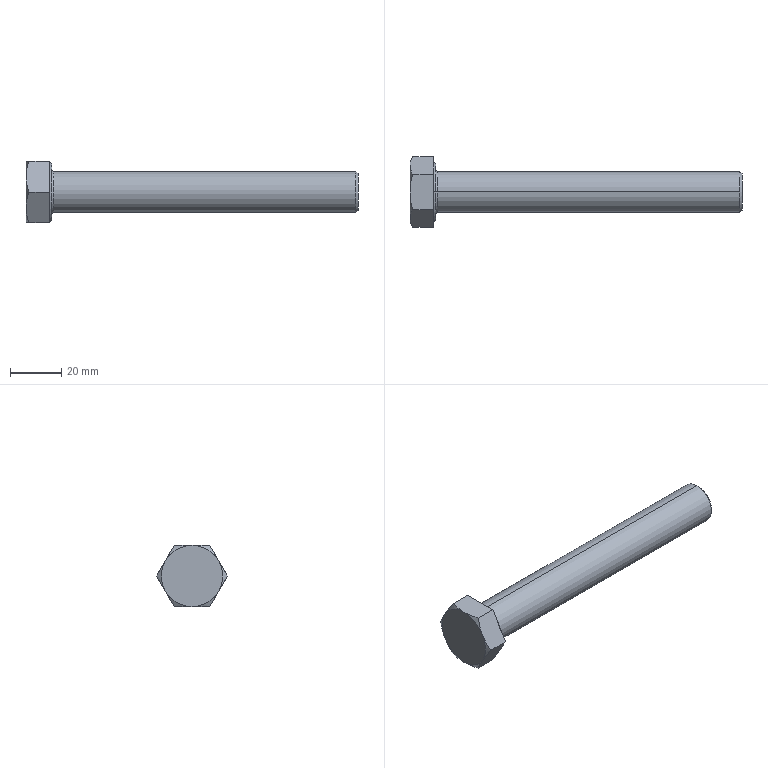Part | SolidWorks | features Chamfer 2, RevCut 2, Revolution 2, Extrusion 1, ICE 1 | 1 solid | 24 faces | box 130 x 27.713 x 24 mm | volume 29026 mm3 | cone 10 | plane 10 | cylinder 2 | torus 2 | commonest cylinder face diameters 16 x2
STEP:
#1=CARTESIAN_POINT('',(10.,0.,11.145));
#2=VERTEX_POINT('',#1);
#3=CARTESIAN_POINT('',(10.,0.,-11.145));
#4=VERTEX_POINT('',#3);
#5=CARTESIAN_POINT('',(10.,0.,0.));
#6=DIRECTION('',(-1.,0.,0.));
#7=DIRECTION('',(0.,0.,1.));
#8=AXIS2_PLACEMENT_3D('',#5,#6,#7);
#9=CIRCLE('',#8,11.145);
#10=EDGE_CURVE('',#2,#4,#9,.T.);
#11=ORIENTED_EDGE('',*,*,#10,.T.);
#12=CARTESIAN_POINT('',(9.2,0.,-11.945));
#13=VERTEX_POINT('',#12);
#14=CARTESIAN_POINT('',(9.2,0.,-11.945));
#15=DIRECTION('',(-0.7071,0.,-0.7071));
#16=VECTOR('',#15,1000.);
#17=LINE('',#14,#16);
#18=EDGE_CURVE('',#4,#13,#17,.T.);
#19=ORIENTED_EDGE('',*,*,#18,.T.);
#20=CARTESIAN_POINT('',(9.2,0.,11.945));
#21=VERTEX_POINT('',#20);
#22=CARTESIAN_POINT('',(9.2,0.,0.));
#23=DIRECTION('',(-1.,0.,0.));
#24=DIRECTION('',(0.,0.,1.));
#25=AXIS2_PLACEMENT_3D('',#22,#23,#24);
#26=CIRCLE('',#25,11.945);
#27=EDGE_CURVE('',#21,#13,#26,.T.);
#28=ORIENTED_EDGE('',*,*,#27,.F.);
#29=CARTESIAN_POINT('',(9.2,0.,11.945));
#30=DIRECTION('',(-0.7071,0.,0.7071));
#31=VECTOR('',#30,1000.);
#32=LINE('',#29,#31);
#33=EDGE_CURVE('',#2,#21,#32,.T.);
#34=ORIENTED_EDGE('',*,*,#33,.F.);
#35=EDGE_LOOP('',(#11,#19,#28,#34));
#36=FACE_OUTER_BOUND('',#35,.T.);
#37=CARTESIAN_POINT('',(9.2,0.,0.));
#38=DIRECTION('',(-1.,0.,0.));
#39=DIRECTION('',(0.,0.,1.));
#40=AXIS2_PLACEMENT_3D('',#37,#38,#39);
#41=CONICAL_SURFACE('',#40,11.945,0.7854);
#42=ADVANCED_FACE('',(#36),#41,.T.);
#43=CARTESIAN_POINT('',(130.,0.,-7.111));
#44=VERTEX_POINT('',#43);
#45=CARTESIAN_POINT('',(130.,0.,7.111));
#46=VERTEX_POINT('',#45);
#47=CARTESIAN_POINT('',(130.,0.,0.));
#48=DIRECTION('',(1.,0.,0.));
#49=DIRECTION('',(0.,0.,1.));
#50=AXIS2_PLACEMENT_3D('',#47,#48,#49);
#51=CIRCLE('',#50,7.111);
#52=EDGE_CURVE('',#44,#46,#51,.T.);
#53=ORIENTED_EDGE('',*,*,#52,.F.);
#54=CARTESIAN_POINT('',(129.111,0.,-8.));
#55=VERTEX_POINT('',#54);
#56=CARTESIAN_POINT('',(129.111,0.,-8.));
#57=DIRECTION('',(-0.7071,0.,-0.7071));
#58=VECTOR('',#57,1000.);
#59=LINE('',#56,#58);
#60=EDGE_CURVE('',#44,#55,#59,.T.);
#61=ORIENTED_EDGE('',*,*,#60,.T.);
#62=CARTESIAN_POINT('',(129.111,0.,8.));
#63=VERTEX_POINT('',#62);
#64=CARTESIAN_POINT('',(129.111,0.,0.));
#65=DIRECTION('',(-1.,0.,0.));
#66=DIRECTION('',(0.,0.,1.));
#67=AXIS2_PLACEMENT_3D('',#64,#65,#66);
#68=CIRCLE('',#67,8.);
#69=EDGE_CURVE('',#63,#55,#68,.T.);
#70=ORIENTED_EDGE('',*,*,#69,.F.);
#71=CARTESIAN_POINT('',(129.111,0.,8.));
#72=DIRECTION('',(-0.7071,0.,0.7071));
#73=VECTOR('',#72,1000.);
#74=LINE('',#71,#73);
#75=EDGE_CURVE('',#46,#63,#74,.T.);
#76=ORIENTED_EDGE('',*,*,#75,.F.);
#77=EDGE_LOOP('',(#53,#61,#70,#76));
#78=FACE_OUTER_BOUND('',#77,.T.);
#79=CARTESIAN_POINT('',(129.111,0.,0.));
#80=DIRECTION('',(-1.,0.,0.));
#81=DIRECTION('',(0.,0.,1.));
#82=AXIS2_PLACEMENT_3D('',#79,#80,#81);
#83=CONICAL_SURFACE('',#82,8.,0.7854);
#84=ADVANCED_FACE('',(#78),#83,.T.);
#85=ORIENTED_EDGE('',*,*,#69,.T.);
#86=CARTESIAN_POINT('',(10.85,0.,-8.));
#87=VERTEX_POINT('',#86);
#88=CARTESIAN_POINT('',(10.,0.,-8.));
#89=DIRECTION('',(-1.,0.,0.));
#90=VECTOR('',#89,1000.);
#91=LINE('',#88,#90);
#92=EDGE_CURVE('',#55,#87,#91,.T.);
#93=ORIENTED_EDGE('',*,*,#92,.T.);
#94=CARTESIAN_POINT('',(10.85,0.,8.));
#95=VERTEX_POINT('',#94);
#96=CARTESIAN_POINT('',(10.85,0.,0.));
#97=DIRECTION('',(-1.,0.,0.));
#98=DIRECTION('',(0.,0.,1.));
#99=AXIS2_PLACEMENT_3D('',#96,#97,#98);
#100=CIRCLE('',#99,8.);
#101=EDGE_CURVE('',#95,#87,#100,.T.);
#102=ORIENTED_EDGE('',*,*,#101,.F.);
#103=CARTESIAN_POINT('',(10.,0.,8.));
#104=DIRECTION('',(-1.,0.,0.));
#105=VECTOR('',#104,1000.);
#106=LINE('',#103,#105);
#107=EDGE_CURVE('',#63,#95,#106,.T.);
#108=ORIENTED_EDGE('',*,*,#107,.F.);
#109=EDGE_LOOP('',(#85,#93,#102,#108));
#110=FACE_OUTER_BOUND('',#109,.T.);
#111=CARTESIAN_POINT('',(10.,0.,0.));
#112=DIRECTION('',(-1.,0.,0.));
#113=DIRECTION('',(0.,0.,1.));
#114=AXIS2_PLACEMENT_3D('',#111,#112,#113);
#115=CYLINDRICAL_SURFACE('',#114,8.);
#116=ADVANCED_FACE('',(#110),#115,.T.);
#117=CARTESIAN_POINT('',(10.,0.,-8.85));
#118=VERTEX_POINT('',#117);
#119=CARTESIAN_POINT('',(10.,0.,8.85));
#120=VERTEX_POINT('',#119);
#121=CARTESIAN_POINT('',(10.,0.,0.));
#122=DIRECTION('',(-1.,0.,0.));
#123=DIRECTION('',(0.,0.,1.));
#124=AXIS2_PLACEMENT_3D('',#121,#122,#123);
#125=CIRCLE('',#124,8.85);
#126=EDGE_CURVE('',#118,#120,#125,.T.);
#127=ORIENTED_EDGE('',*,*,#126,.F.);
#128=CARTESIAN_POINT('',(10.85,0.,-8.85));
#129=DIRECTION('',(0.,1.,0.));
#130=DIRECTION('',(0.,0.,1.));
#131=AXIS2_PLACEMENT_3D('',#128,#129,#130);
#132=CIRCLE('',#131,0.85);
#133=EDGE_CURVE('',#118,#87,#132,.T.);
#134=ORIENTED_EDGE('',*,*,#133,.T.);
#135=CARTESIAN_POINT('',(10.85,0.,0.));
#136=DIRECTION('',(-1.,0.,0.));
#137=DIRECTION('',(0.,0.,1.));
#138=AXIS2_PLACEMENT_3D('',#135,#136,#137);
#139=CIRCLE('',#138,8.);
#140=EDGE_CURVE('',#87,#95,#139,.T.);
#141=ORIENTED_EDGE('',*,*,#140,.T.);
#142=CARTESIAN_POINT('',(10.85,0.,8.85));
#143=DIRECTION('',(0.,-1.,0.));
#144=DIRECTION('',(0.,0.,-1.));
#145=AXIS2_PLACEMENT_3D('',#142,#143,#144);
#146=CIRCLE('',#145,0.85);
#147=EDGE_CURVE('',#120,#95,#146,.T.);
#148=ORIENTED_EDGE('',*,*,#147,.F.);
#149=EDGE_LOOP('',(#127,#134,#141,#148));
#150=FACE_OUTER_BOUND('',#149,.T.);
#151=CARTESIAN_POINT('',(10.85,0.,0.));
#152=DIRECTION('',(-1.,0.,0.));
#153=DIRECTION('',(0.,0.,1.));
#154=AXIS2_PLACEMENT_3D('',#151,#152,#153);
#155=TOROIDAL_SURFACE('',#154,8.85,0.85);
#156=ADVANCED_FACE('',(#150),#155,.F.);
#157=CARTESIAN_POINT('',(10.,0.,0.));
#158=DIRECTION('',(-1.,0.,0.));
#159=DIRECTION('',(0.,0.,1.));
#160=AXIS2_PLACEMENT_3D('',#157,#158,#159);
#161=CIRCLE('',#160,8.85);
#162=EDGE_CURVE('',#120,#118,#161,.T.);
#163=ORIENTED_EDGE('',*,*,#162,.T.);
#164=ORIENTED_EDGE('',*,*,#126,.T.);
#165=EDGE_LOOP('',(#163,#164));
#166=FACE_BOUND('',#165,.T.);
#167=ORIENTED_EDGE('',*,*,#10,.F.);
#168=CARTESIAN_POINT('',(10.,0.,0.));
#169=DIRECTION('',(-1.,0.,0.));
#170=DIRECTION('',(0.,0.,1.));
#171=AXIS2_PLACEMENT_3D('',#168,#169,#170);
#172=CIRCLE('',#171,11.145);
#173=EDGE_CURVE('',#4,#2,#172,.T.);
#174=ORIENTED_EDGE('',*,*,#173,.F.);
#175=EDGE_LOOP('',(#167,#174));
#176=FACE_OUTER_BOUND('',#175,.T.);
#177=CARTESIAN_POINT('',(10.,6.928,-12.));
#178=DIRECTION('',(1.,0.,0.));
#179=DIRECTION('',(0.,0.,-1.));
#180=AXIS2_PLACEMENT_3D('',#177,#178,#179);
#181=PLANE('',#180);
#182=ADVANCED_FACE('',(#166,#176),#181,.T.);
#183=ORIENTED_EDGE('',*,*,#133,.F.);
#184=ORIENTED_EDGE('',*,*,#162,.F.);
#185=ORIENTED_EDGE('',*,*,#147,.T.);
#186=ORIENTED_EDGE('',*,*,#101,.T.);
#187=EDGE_LOOP('',(#183,#184,#185,#186));
#188=FACE_OUTER_BOUND('',#187,.T.);
#189=CARTESIAN_POINT('',(10.85,0.,0.));
#190=DIRECTION('',(-1.,0.,0.));
#191=DIRECTION('',(0.,0.,1.));
#192=AXIS2_PLACEMENT_3D('',#189,#190,#191);
#193=TOROIDAL_SURFACE('',#192,8.85,0.85);
#194=ADVANCED_FACE('',(#188),#193,.F.);
#195=CARTESIAN_POINT('',(130.,0.,0.));
#196=DIRECTION('',(1.,0.,0.));
#197=DIRECTION('',(0.,0.,1.));
#198=AXIS2_PLACEMENT_3D('',#195,#196,#197);
#199=CIRCLE('',#198,7.111);
#200=EDGE_CURVE('',#46,#44,#199,.T.);
#201=ORIENTED_EDGE('',*,*,#200,.T.);
#202=ORIENTED_EDGE('',*,*,#52,.T.);
#203=EDGE_LOOP('',(#201,#202));
#204=FACE_OUTER_BOUND('',#203,.T.);
#205=CARTESIAN_POINT('',(130.,8.,0.));
#206=DIRECTION('',(-1.,0.,0.));
#207=DIRECTION('',(0.,0.,1.));
#208=AXIS2_PLACEMENT_3D('',#205,#206,#207);
#209=PLANE('',#208);
#210=ADVANCED_FACE('',(#204),#209,.F.);
#211=ORIENTED_EDGE('',*,*,#92,.F.);
#212=CARTESIAN_POINT('',(129.111,0.,0.));
#213=DIRECTION('',(-1.,0.,0.));
#214=DIRECTION('',(0.,0.,1.));
#215=AXIS2_PLACEMENT_3D('',#212,#213,#214);
#216=CIRCLE('',#215,8.);
#217=EDGE_CURVE('',#55,#63,#216,.T.);
#218=ORIENTED_EDGE('',*,*,#217,.T.);
#219=ORIENTED_EDGE('',*,*,#107,.T.);
#220=ORIENTED_EDGE('',*,*,#140,.F.);
#221=EDGE_LOOP('',(#211,#218,#219,#220));
#222=FACE_OUTER_BOUND('',#221,.T.);
#223=CARTESIAN_POINT('',(10.,0.,0.));
#224=DIRECTION('',(-1.,0.,0.));
#225=DIRECTION('',(0.,0.,1.));
#226=AXIS2_PLACEMENT_3D('',#223,#224,#225);
#227=CYLINDRICAL_SURFACE('',#226,8.);
#228=ADVANCED_FACE('',(#222),#227,.T.);
#229=ORIENTED_EDGE('',*,*,#60,.F.);
#230=ORIENTED_EDGE('',*,*,#200,.F.);
#231=ORIENTED_EDGE('',*,*,#75,.T.);
#232=ORIENTED_EDGE('',*,*,#217,.F.);
#233=EDGE_LOOP('',(#229,#230,#231,#232));
#234=FACE_OUTER_BOUND('',#233,.T.);
#235=CARTESIAN_POINT('',(129.111,0.,0.));
#236=DIRECTION('',(-1.,0.,0.));
#237=DIRECTION('',(0.,0.,1.));
#238=AXIS2_PLACEMENT_3D('',#235,#236,#237);
#239=CONICAL_SURFACE('',#238,8.,0.7854);
#240=ADVANCED_FACE('',(#234),#239,.T.);
#241=ORIENTED_EDGE('',*,*,#27,.T.);
#242=CARTESIAN_POINT('',(9.2,0.,0.));
#243=DIRECTION('',(-1.,0.,0.));
#244=DIRECTION('',(0.,0.,1.));
#245=AXIS2_PLACEMENT_3D('',#242,#243,#244);
#246=CIRCLE('',#245,11.945);
#247=EDGE_CURVE('',#13,#21,#246,.T.);
#248=ORIENTED_EDGE('',*,*,#247,.T.);
#249=EDGE_LOOP('',(#241,#248));
#250=FACE_BOUND('',#249,.T.);
#251=CARTESIAN_POINT('',(9.2,-6.928,-12.));
#252=VERTEX_POINT('',#251);
#253=CARTESIAN_POINT('',(9.2,6.928,-12.));
#254=VERTEX_POINT('',#253);
#255=CARTESIAN_POINT('',(9.2,-6.928,-12.));
#256=DIRECTION('',(0.,1.,0.));
#257=VECTOR('',#256,1000.);
#258=LINE('',#255,#257);
#259=EDGE_CURVE('',#252,#254,#258,.T.);
#260=ORIENTED_EDGE('',*,*,#259,.T.);
#261=CARTESIAN_POINT('',(9.2,13.856,0.));
#262=VERTEX_POINT('',#261);
#263=CARTESIAN_POINT('',(9.2,6.928,-12.));
#264=DIRECTION('',(0.,0.5,0.866));
#265=VECTOR('',#264,1000.);
#266=LINE('',#263,#265);
#267=EDGE_CURVE('',#254,#262,#266,.T.);
#268=ORIENTED_EDGE('',*,*,#267,.T.);
#269=CARTESIAN_POINT('',(9.2,6.928,12.));
#270=VERTEX_POINT('',#269);
#271=CARTESIAN_POINT('',(9.2,13.856,0.));
#272=DIRECTION('',(0.,-0.5,0.866));
#273=VECTOR('',#272,1000.);
#274=LINE('',#271,#273);
#275=EDGE_CURVE('',#262,#270,#274,.T.);
#276=ORIENTED_EDGE('',*,*,#275,.T.);
#277=CARTESIAN_POINT('',(9.2,-6.928,12.));
#278=VERTEX_POINT('',#277);
#279=CARTESIAN_POINT('',(9.2,6.928,12.));
#280=DIRECTION('',(0.,-1.,0.));
#281=VECTOR('',#280,1000.);
#282=LINE('',#279,#281);
#283=EDGE_CURVE('',#270,#278,#282,.T.);
#284=ORIENTED_EDGE('',*,*,#283,.T.);
#285=CARTESIAN_POINT('',(9.2,-13.856,0.));
#286=VERTEX_POINT('',#285);
#287=CARTESIAN_POINT('',(9.2,-6.928,12.));
#288=DIRECTION('',(0.,-0.5,-0.866));
#289=VECTOR('',#288,1000.);
#290=LINE('',#287,#289);
#291=EDGE_CURVE('',#278,#286,#290,.T.);
#292=ORIENTED_EDGE('',*,*,#291,.T.);
#293=CARTESIAN_POINT('',(9.2,-13.856,0.));
#294=DIRECTION('',(0.,0.5,-0.866));
#295=VECTOR('',#294,1000.);
#296=LINE('',#293,#295);
#297=EDGE_CURVE('',#286,#252,#296,.T.);
#298=ORIENTED_EDGE('',*,*,#297,.T.);
#299=EDGE_LOOP('',(#260,#268,#276,#284,#292,#298));
#300=FACE_OUTER_BOUND('',#299,.T.);
#301=CARTESIAN_POINT('',(9.2,-11.945,0.));
#302=DIRECTION('',(1.,0.,0.));
#303=DIRECTION('',(0.,0.,-1.));
#304=AXIS2_PLACEMENT_3D('',#301,#302,#303);
#305=PLANE('',#304);
#306=ADVANCED_FACE('',(#250,#300),#305,.T.);
#307=ORIENTED_EDGE('',*,*,#18,.F.);
#308=ORIENTED_EDGE('',*,*,#173,.T.);
#309=ORIENTED_EDGE('',*,*,#33,.T.);
#310=ORIENTED_EDGE('',*,*,#247,.F.);
#311=EDGE_LOOP('',(#307,#308,#309,#310));
#312=FACE_OUTER_BOUND('',#311,.T.);
#313=CARTESIAN_POINT('',(9.2,0.,0.));
#314=DIRECTION('',(-1.,0.,0.));
#315=DIRECTION('',(0.,0.,1.));
#316=AXIS2_PLACEMENT_3D('',#313,#314,#315);
#317=CONICAL_SURFACE('',#316,11.945,0.7854);
#318=ADVANCED_FACE('',(#312),#317,.T.);
#319=CARTESIAN_POINT('',(0.,0.,-12.));
#320=VERTEX_POINT('',#319);
#321=CARTESIAN_POINT('',(0.,10.392,-6.));
#322=VERTEX_POINT('',#321);
#323=CARTESIAN_POINT('',(0.,0.,0.));
#324=DIRECTION('',(1.,0.,0.));
#325=DIRECTION('',(0.,0.,-1.));
#326=AXIS2_PLACEMENT_3D('',#323,#324,#325);
#327=CIRCLE('',#326,12.);
#328=EDGE_CURVE('',#320,#322,#327,.T.);
#329=ORIENTED_EDGE('',*,*,#328,.F.);
#330=CARTESIAN_POINT('',(0.,-10.392,-6.));
#331=VERTEX_POINT('',#330);
#332=CARTESIAN_POINT('',(0.,0.,0.));
#333=DIRECTION('',(1.,0.,0.));
#334=DIRECTION('',(0.,0.,-1.));
#335=AXIS2_PLACEMENT_3D('',#332,#333,#334);
#336=CIRCLE('',#335,12.);
#337=EDGE_CURVE('',#331,#320,#336,.T.);
#338=ORIENTED_EDGE('',*,*,#337,.F.);
#339=CARTESIAN_POINT('',(0.,-10.392,6.));
#340=VERTEX_POINT('',#339);
#341=CARTESIAN_POINT('',(0.,0.,0.));
#342=DIRECTION('',(1.,0.,0.));
#343=DIRECTION('',(0.,0.,-1.));
#344=AXIS2_PLACEMENT_3D('',#341,#342,#343);
#345=CIRCLE('',#344,12.);
#346=EDGE_CURVE('',#340,#331,#345,.T.);
#347=ORIENTED_EDGE('',*,*,#346,.F.);
#348=CARTESIAN_POINT('',(0.,0.,12.));
#349=VERTEX_POINT('',#348);
#350=CARTESIAN_POINT('',(0.,0.,0.));
#351=DIRECTION('',(1.,0.,0.));
#352=DIRECTION('',(0.,0.,-1.));
#353=AXIS2_PLACEMENT_3D('',#350,#351,#352);
#354=CIRCLE('',#353,12.);
#355=EDGE_CURVE('',#349,#340,#354,.T.);
#356=ORIENTED_EDGE('',*,*,#355,.F.);
#357=CARTESIAN_POINT('',(0.,10.392,6.));
#358=VERTEX_POINT('',#357);
#359=CARTESIAN_POINT('',(0.,0.,0.));
#360=DIRECTION('',(-1.,0.,0.));
#361=DIRECTION('',(0.,0.,1.));
#362=AXIS2_PLACEMENT_3D('',#359,#360,#361);
#363=CIRCLE('',#362,12.);
#364=EDGE_CURVE('',#349,#358,#363,.T.);
#365=ORIENTED_EDGE('',*,*,#364,.T.);
#366=CARTESIAN_POINT('',(0.,0.,0.));
#367=DIRECTION('',(1.,0.,0.));
#368=DIRECTION('',(0.,0.,-1.));
#369=AXIS2_PLACEMENT_3D('',#366,#367,#368);
#370=CIRCLE('',#369,12.);
#371=EDGE_CURVE('',#322,#358,#370,.T.);
#372=ORIENTED_EDGE('',*,*,#371,.F.);
#373=EDGE_LOOP('',(#329,#338,#347,#356,#365,#372));
#374=FACE_OUTER_BOUND('',#373,.T.);
#375=CARTESIAN_POINT('',(0.,6.928,-12.));
#376=DIRECTION('',(1.,0.,0.));
#377=DIRECTION('',(0.,0.,-1.));
#378=AXIS2_PLACEMENT_3D('',#375,#376,#377);
#379=PLANE('',#378);
#380=ADVANCED_FACE('',(#374),#379,.F.);
#381=CARTESIAN_POINT('',(1.072,6.928,-12.));
#382=VERTEX_POINT('',#381);
#383=CARTESIAN_POINT('',(0.,10.392,-6.));
#384=CARTESIAN_POINT('',(0.,10.098,-6.509));
#385=CARTESIAN_POINT('',(0.02533,9.803,-7.021));
#386=CARTESIAN_POINT('',(0.1234,9.219,-8.033));
#387=CARTESIAN_POINT('',(0.196,8.929,-8.535));
#388=CARTESIAN_POINT('',(0.476,8.063,-10.034));
#389=CARTESIAN_POINT('',(0.7454,7.493,-11.021));
#390=CARTESIAN_POINT('',(1.072,6.928,-12.));
#391=B_SPLINE_CURVE_WITH_KNOTS('',3,(#383,#384,#385,#386,#387,#388,#389,#390),.UNSPECIFIED.,.F.,.F.,(4,2,2,4),(0.00701,0.008756,0.0105,0.01399),.UNSPECIFIED.);
#392=EDGE_CURVE('',#322,#382,#391,.T.);
#393=ORIENTED_EDGE('',*,*,#392,.T.);
#394=CARTESIAN_POINT('',(1.072,6.928,-12.));
#395=CARTESIAN_POINT('',(0.7484,5.808,-12.));
#396=CARTESIAN_POINT('',(0.4791,4.673,-12.));
#397=CARTESIAN_POINT('',(0.1974,2.937,-12.));
#398=CARTESIAN_POINT('',(0.1238,2.353,-12.));
#399=CARTESIAN_POINT('',(0.0249,1.173,-12.));
#400=CARTESIAN_POINT('',(0.,0.5858,-12.));
#401=CARTESIAN_POINT('',(0.,0.,-12.));
#402=B_SPLINE_CURVE_WITH_KNOTS('',3,(#394,#395,#396,#397,#398,#399,#400,#401),.UNSPECIFIED.,.F.,.F.,(4,2,2,4),(0.005049,0.008547,0.0103,0.01204),.UNSPECIFIED.);
#403=EDGE_CURVE('',#382,#320,#402,.T.);
#404=ORIENTED_EDGE('',*,*,#403,.T.);
#405=ORIENTED_EDGE('',*,*,#328,.T.);
#406=EDGE_LOOP('',(#393,#404,#405));
#407=FACE_OUTER_BOUND('',#406,.T.);
#408=CARTESIAN_POINT('',(0.,0.,0.));
#409=DIRECTION('',(1.,0.,0.));
#410=DIRECTION('',(0.,0.,1.));
#411=AXIS2_PLACEMENT_3D('',#408,#409,#410);
#412=CONICAL_SURFACE('',#411,12.,1.047);
#413=ADVANCED_FACE('',(#407),#412,.T.);
#414=CARTESIAN_POINT('',(1.072,13.856,0.));
#415=VERTEX_POINT('',#414);
#416=CARTESIAN_POINT('',(0.,10.392,6.));
#417=CARTESIAN_POINT('',(0.,10.686,5.491));
#418=CARTESIAN_POINT('',(0.02533,10.982,4.979));
#419=CARTESIAN_POINT('',(0.1234,11.566,3.967));
#420=CARTESIAN_POINT('',(0.196,11.856,3.465));
#421=CARTESIAN_POINT('',(0.476,12.721,1.966));
#422=CARTESIAN_POINT('',(0.7454,13.291,0.9791));
#423=CARTESIAN_POINT('',(1.072,13.856,0.));
#424=B_SPLINE_CURVE_WITH_KNOTS('',3,(#416,#417,#418,#419,#420,#421,#422,#423),.UNSPECIFIED.,.F.,.F.,(4,2,2,4),(0.00701,0.008756,0.0105,0.01399),.UNSPECIFIED.);
#425=EDGE_CURVE('',#358,#415,#424,.T.);
#426=ORIENTED_EDGE('',*,*,#425,.T.);
#427=CARTESIAN_POINT('',(1.072,13.856,0.));
#428=CARTESIAN_POINT('',(0.7446,13.29,-0.9815));
#429=CARTESIAN_POINT('',(0.4751,12.719,-1.97));
#430=CARTESIAN_POINT('',(0.1021,11.565,-3.968));
#431=CARTESIAN_POINT('',(0.,10.982,-4.978));
#432=CARTESIAN_POINT('',(0.,10.392,-6.));
#433=B_SPLINE_CURVE_WITH_KNOTS('',3,(#427,#428,#429,#430,#431,#432),.UNSPECIFIED.,.F.,.F.,(4,2,4),(0.000000238,0.003505,0.00701),.UNSPECIFIED.);
#434=EDGE_CURVE('',#415,#322,#433,.T.);
#435=ORIENTED_EDGE('',*,*,#434,.T.);
#436=ORIENTED_EDGE('',*,*,#371,.T.);
#437=EDGE_LOOP('',(#426,#435,#436));
#438=FACE_OUTER_BOUND('',#437,.T.);
#439=CARTESIAN_POINT('',(0.,0.,0.));
#440=DIRECTION('',(1.,0.,0.));
#441=DIRECTION('',(0.,0.,1.));
#442=AXIS2_PLACEMENT_3D('',#439,#440,#441);
#443=CONICAL_SURFACE('',#442,12.,1.047);
#444=ADVANCED_FACE('',(#438),#443,.T.);
#445=CARTESIAN_POINT('',(1.072,6.928,12.));
#446=VERTEX_POINT('',#445);
#447=CARTESIAN_POINT('',(1.072,6.928,12.));
#448=CARTESIAN_POINT('',(0.7446,7.495,11.018));
#449=CARTESIAN_POINT('',(0.4751,8.066,10.03));
#450=CARTESIAN_POINT('',(0.1021,9.219,8.032));
#451=CARTESIAN_POINT('',(0.,9.802,7.022));
#452=CARTESIAN_POINT('',(0.,10.392,6.));
#453=B_SPLINE_CURVE_WITH_KNOTS('',3,(#447,#448,#449,#450,#451,#452),.UNSPECIFIED.,.F.,.F.,(4,2,4),(0.000000238,0.003505,0.00701),.UNSPECIFIED.);
#454=EDGE_CURVE('',#446,#358,#453,.T.);
#455=ORIENTED_EDGE('',*,*,#454,.T.);
#456=ORIENTED_EDGE('',*,*,#364,.F.);
#457=CARTESIAN_POINT('',(0.,0.,12.));
#458=CARTESIAN_POINT('',(0.,0.5858,12.));
#459=CARTESIAN_POINT('',(0.0249,1.173,12.));
#460=CARTESIAN_POINT('',(0.1238,2.353,12.));
#461=CARTESIAN_POINT('',(0.1974,2.937,12.));
#462=CARTESIAN_POINT('',(0.4791,4.673,12.));
#463=CARTESIAN_POINT('',(0.7484,5.808,12.));
#464=CARTESIAN_POINT('',(1.072,6.928,12.));
#465=B_SPLINE_CURVE_WITH_KNOTS('',3,(#457,#458,#459,#460,#461,#462,#463,#464),.UNSPECIFIED.,.F.,.F.,(4,2,2,4),(0.0194,0.02115,0.0229,0.02641),.UNSPECIFIED.);
#466=EDGE_CURVE('',#349,#446,#465,.T.);
#467=ORIENTED_EDGE('',*,*,#466,.T.);
#468=EDGE_LOOP('',(#455,#456,#467));
#469=FACE_OUTER_BOUND('',#468,.T.);
#470=CARTESIAN_POINT('',(0.,0.,0.));
#471=DIRECTION('',(1.,0.,0.));
#472=DIRECTION('',(0.,0.,1.));
#473=AXIS2_PLACEMENT_3D('',#470,#471,#472);
#474=CONICAL_SURFACE('',#473,12.,1.047);
#475=ADVANCED_FACE('',(#469),#474,.T.);
#476=CARTESIAN_POINT('',(1.072,-6.928,12.));
#477=VERTEX_POINT('',#476);
#478=CARTESIAN_POINT('',(1.072,-6.928,12.));
#479=CARTESIAN_POINT('',(0.7465,-5.801,12.));
#480=CARTESIAN_POINT('',(0.4737,-4.647,12.));
#481=CARTESIAN_POINT('',(0.1006,-2.334,12.));
#482=CARTESIAN_POINT('',(0.,-1.171,12.));
#483=CARTESIAN_POINT('',(0.,0.,12.));
#484=B_SPLINE_CURVE_WITH_KNOTS('',3,(#478,#479,#480,#481,#482,#483),.UNSPECIFIED.,.F.,.F.,(4,2,4),(0.01239,0.01589,0.0194),.UNSPECIFIED.);
#485=EDGE_CURVE('',#477,#349,#484,.T.);
#486=ORIENTED_EDGE('',*,*,#485,.T.);
#487=ORIENTED_EDGE('',*,*,#355,.T.);
#488=CARTESIAN_POINT('',(0.,-10.392,6.));
#489=CARTESIAN_POINT('',(0.,-10.098,6.509));
#490=CARTESIAN_POINT('',(0.02533,-9.803,7.021));
#491=CARTESIAN_POINT('',(0.1234,-9.219,8.033));
#492=CARTESIAN_POINT('',(0.196,-8.929,8.535));
#493=CARTESIAN_POINT('',(0.476,-8.063,10.034));
#494=CARTESIAN_POINT('',(0.7454,-7.493,11.021));
#495=CARTESIAN_POINT('',(1.072,-6.928,12.));
#496=B_SPLINE_CURVE_WITH_KNOTS('',3,(#488,#489,#490,#491,#492,#493,#494,#495),.UNSPECIFIED.,.F.,.F.,(4,2,2,4),(0.00701,0.008756,0.0105,0.01399),.UNSPECIFIED.);
#497=EDGE_CURVE('',#340,#477,#496,.T.);
#498=ORIENTED_EDGE('',*,*,#497,.T.);
#499=EDGE_LOOP('',(#486,#487,#498));
#500=FACE_OUTER_BOUND('',#499,.T.);
#501=CARTESIAN_POINT('',(0.,0.,0.));
#502=DIRECTION('',(1.,0.,0.));
#503=DIRECTION('',(0.,0.,1.));
#504=AXIS2_PLACEMENT_3D('',#501,#502,#503);
#505=CONICAL_SURFACE('',#504,12.,1.047);
#506=ADVANCED_FACE('',(#500),#505,.T.);
#507=CARTESIAN_POINT('',(1.072,-6.928,-12.));
#508=VERTEX_POINT('',#507);
#509=CARTESIAN_POINT('',(0.,0.,-12.));
#510=CARTESIAN_POINT('',(0.,-1.171,-12.));
#511=CARTESIAN_POINT('',(0.1006,-2.334,-12.));
#512=CARTESIAN_POINT('',(0.4737,-4.647,-12.));
#513=CARTESIAN_POINT('',(0.7465,-5.801,-12.));
#514=CARTESIAN_POINT('',(1.072,-6.928,-12.));
#515=B_SPLINE_CURVE_WITH_KNOTS('',3,(#509,#510,#511,#512,#513,#514),.UNSPECIFIED.,.F.,.F.,(4,2,4),(0.01204,0.01554,0.01904),.UNSPECIFIED.);
#516=EDGE_CURVE('',#320,#508,#515,.T.);
#517=ORIENTED_EDGE('',*,*,#516,.T.);
#518=CARTESIAN_POINT('',(1.072,-6.928,-12.));
#519=CARTESIAN_POINT('',(0.7446,-7.495,-11.018));
#520=CARTESIAN_POINT('',(0.4751,-8.066,-10.03));
#521=CARTESIAN_POINT('',(0.1021,-9.219,-8.032));
#522=CARTESIAN_POINT('',(0.,-9.802,-7.022));
#523=CARTESIAN_POINT('',(0.,-10.392,-6.));
#524=B_SPLINE_CURVE_WITH_KNOTS('',3,(#518,#519,#520,#521,#522,#523),.UNSPECIFIED.,.F.,.F.,(4,2,4),(0.000000238,0.003505,0.00701),.UNSPECIFIED.);
#525=EDGE_CURVE('',#508,#331,#524,.T.);
#526=ORIENTED_EDGE('',*,*,#525,.T.);
#527=ORIENTED_EDGE('',*,*,#337,.T.);
#528=EDGE_LOOP('',(#517,#526,#527));
#529=FACE_OUTER_BOUND('',#528,.T.);
#530=CARTESIAN_POINT('',(0.,0.,0.));
#531=DIRECTION('',(1.,0.,0.));
#532=DIRECTION('',(0.,0.,1.));
#533=AXIS2_PLACEMENT_3D('',#530,#531,#532);
#534=CONICAL_SURFACE('',#533,12.,1.047);
#535=ADVANCED_FACE('',(#529),#534,.T.);
#536=CARTESIAN_POINT('',(1.072,-13.856,0.));
#537=VERTEX_POINT('',#536);
#538=CARTESIAN_POINT('',(1.072,-13.856,0.));
#539=CARTESIAN_POINT('',(0.7446,-13.29,0.9815));
#540=CARTESIAN_POINT('',(0.4751,-12.719,1.97));
#541=CARTESIAN_POINT('',(0.1021,-11.565,3.968));
#542=CARTESIAN_POINT('',(0.,-10.982,4.978));
#543=CARTESIAN_POINT('',(0.,-10.392,6.));
#544=B_SPLINE_CURVE_WITH_KNOTS('',3,(#538,#539,#540,#541,#542,#543),.UNSPECIFIED.,.F.,.F.,(4,2,4),(0.000000238,0.003505,0.00701),.UNSPECIFIED.);
#545=EDGE_CURVE('',#537,#340,#544,.T.);
#546=ORIENTED_EDGE('',*,*,#545,.T.);
#547=ORIENTED_EDGE('',*,*,#346,.T.);
#548=CARTESIAN_POINT('',(0.,-10.392,-6.));
#549=CARTESIAN_POINT('',(0.,-10.686,-5.491));
#550=CARTESIAN_POINT('',(0.02533,-10.982,-4.979));
#551=CARTESIAN_POINT('',(0.1234,-11.566,-3.967));
#552=CARTESIAN_POINT('',(0.196,-11.856,-3.465));
#553=CARTESIAN_POINT('',(0.476,-12.721,-1.966));
#554=CARTESIAN_POINT('',(0.7454,-13.291,-0.9791));
#555=CARTESIAN_POINT('',(1.072,-13.856,0.));
#556=B_SPLINE_CURVE_WITH_KNOTS('',3,(#548,#549,#550,#551,#552,#553,#554,#555),.UNSPECIFIED.,.F.,.F.,(4,2,2,4),(0.00701,0.008756,0.0105,0.01399),.UNSPECIFIED.);
#557=EDGE_CURVE('',#331,#537,#556,.T.);
#558=ORIENTED_EDGE('',*,*,#557,.T.);
#559=EDGE_LOOP('',(#546,#547,#558));
#560=FACE_OUTER_BOUND('',#559,.T.);
#561=CARTESIAN_POINT('',(0.,0.,0.));
#562=DIRECTION('',(1.,0.,0.));
#563=DIRECTION('',(0.,0.,1.));
#564=AXIS2_PLACEMENT_3D('',#561,#562,#563);
#565=CONICAL_SURFACE('',#564,12.,1.047);
#566=ADVANCED_FACE('',(#560),#565,.T.);
#567=ORIENTED_EDGE('',*,*,#297,.F.);
#568=CARTESIAN_POINT('',(10.,-13.856,0.));
#569=DIRECTION('',(-1.,0.,0.));
#570=VECTOR('',#569,1000.);
#571=LINE('',#568,#570);
#572=EDGE_CURVE('',#286,#537,#571,.T.);
#573=ORIENTED_EDGE('',*,*,#572,.T.);
#574=ORIENTED_EDGE('',*,*,#557,.F.);
#575=ORIENTED_EDGE('',*,*,#525,.F.);
#576=CARTESIAN_POINT('',(10.,-6.928,-12.));
#577=DIRECTION('',(-1.,0.,0.));
#578=VECTOR('',#577,1000.);
#579=LINE('',#576,#578);
#580=EDGE_CURVE('',#252,#508,#579,.T.);
#581=ORIENTED_EDGE('',*,*,#580,.F.);
#582=EDGE_LOOP('',(#567,#573,#574,#575,#581));
#583=FACE_OUTER_BOUND('',#582,.T.);
#584=CARTESIAN_POINT('',(10.,-13.856,0.));
#585=DIRECTION('',(0.,0.866,0.5));
#586=DIRECTION('',(0.,-0.5,0.866));
#587=AXIS2_PLACEMENT_3D('',#584,#585,#586);
#588=PLANE('',#587);
#589=ADVANCED_FACE('',(#583),#588,.F.);
#590=ORIENTED_EDGE('',*,*,#291,.F.);
#591=CARTESIAN_POINT('',(10.,-6.928,12.));
#592=DIRECTION('',(-1.,0.,0.));
#593=VECTOR('',#592,1000.);
#594=LINE('',#591,#593);
#595=EDGE_CURVE('',#278,#477,#594,.T.);
#596=ORIENTED_EDGE('',*,*,#595,.T.);
#597=ORIENTED_EDGE('',*,*,#497,.F.);
#598=ORIENTED_EDGE('',*,*,#545,.F.);
#599=ORIENTED_EDGE('',*,*,#572,.F.);
#600=EDGE_LOOP('',(#590,#596,#597,#598,#599));
#601=FACE_OUTER_BOUND('',#600,.T.);
#602=CARTESIAN_POINT('',(10.,-6.928,12.));
#603=DIRECTION('',(0.,0.866,-0.5));
#604=DIRECTION('',(0.,0.5,0.866));
#605=AXIS2_PLACEMENT_3D('',#602,#603,#604);
#606=PLANE('',#605);
#607=ADVANCED_FACE('',(#601),#606,.F.);
#608=ORIENTED_EDGE('',*,*,#283,.F.);
#609=CARTESIAN_POINT('',(10.,6.928,12.));
#610=DIRECTION('',(-1.,0.,0.));
#611=VECTOR('',#610,1000.);
#612=LINE('',#609,#611);
#613=EDGE_CURVE('',#270,#446,#612,.T.);
#614=ORIENTED_EDGE('',*,*,#613,.T.);
#615=ORIENTED_EDGE('',*,*,#466,.F.);
#616=ORIENTED_EDGE('',*,*,#485,.F.);
#617=ORIENTED_EDGE('',*,*,#595,.F.);
#618=EDGE_LOOP('',(#608,#614,#615,#616,#617));
#619=FACE_OUTER_BOUND('',#618,.T.);
#620=CARTESIAN_POINT('',(10.,6.928,12.));
#621=DIRECTION('',(0.,0.,-1.));
#622=DIRECTION('',(0.,1.,0.));
#623=AXIS2_PLACEMENT_3D('',#620,#621,#622);
#624=PLANE('',#623);
#625=ADVANCED_FACE('',(#619),#624,.F.);
#626=ORIENTED_EDGE('',*,*,#275,.F.);
#627=CARTESIAN_POINT('',(10.,13.856,0.));
#628=DIRECTION('',(-1.,0.,0.));
#629=VECTOR('',#628,1000.);
#630=LINE('',#627,#629);
#631=EDGE_CURVE('',#262,#415,#630,.T.);
#632=ORIENTED_EDGE('',*,*,#631,.T.);
#633=ORIENTED_EDGE('',*,*,#425,.F.);
#634=ORIENTED_EDGE('',*,*,#454,.F.);
#635=ORIENTED_EDGE('',*,*,#613,.F.);
#636=EDGE_LOOP('',(#626,#632,#633,#634,#635));
#637=FACE_OUTER_BOUND('',#636,.T.);
#638=CARTESIAN_POINT('',(10.,13.856,0.));
#639=DIRECTION('',(0.,-0.866,-0.5));
#640=DIRECTION('',(0.,0.5,-0.866));
#641=AXIS2_PLACEMENT_3D('',#638,#639,#640);
#642=PLANE('',#641);
#643=ADVANCED_FACE('',(#637),#642,.F.);
#644=ORIENTED_EDGE('',*,*,#267,.F.);
#645=CARTESIAN_POINT('',(10.,6.928,-12.));
#646=DIRECTION('',(-1.,0.,0.));
#647=VECTOR('',#646,1000.);
#648=LINE('',#645,#647);
#649=EDGE_CURVE('',#254,#382,#648,.T.);
#650=ORIENTED_EDGE('',*,*,#649,.T.);
#651=ORIENTED_EDGE('',*,*,#392,.F.);
#652=ORIENTED_EDGE('',*,*,#434,.F.);
#653=ORIENTED_EDGE('',*,*,#631,.F.);
#654=EDGE_LOOP('',(#644,#650,#651,#652,#653));
#655=FACE_OUTER_BOUND('',#654,.T.);
#656=CARTESIAN_POINT('',(10.,6.928,-12.));
#657=DIRECTION('',(0.,-0.866,0.5));
#658=DIRECTION('',(0.,-0.5,-0.866));
#659=AXIS2_PLACEMENT_3D('',#656,#657,#658);
#660=PLANE('',#659);
#661=ADVANCED_FACE('',(#655),#660,.F.);
#662=ORIENTED_EDGE('',*,*,#259,.F.);
#663=ORIENTED_EDGE('',*,*,#580,.T.);
#664=ORIENTED_EDGE('',*,*,#516,.F.);
#665=ORIENTED_EDGE('',*,*,#403,.F.);
#666=ORIENTED_EDGE('',*,*,#649,.F.);
#667=EDGE_LOOP('',(#662,#663,#664,#665,#666));
#668=FACE_OUTER_BOUND('',#667,.T.);
#669=CARTESIAN_POINT('',(10.,-6.928,-12.));
#670=DIRECTION('',(0.,0.,1.));
#671=DIRECTION('',(0.,-1.,0.));
#672=AXIS2_PLACEMENT_3D('',#669,#670,#671);
#673=PLANE('',#672);
#674=ADVANCED_FACE('',(#668),#673,.F.);
#675=CLOSED_SHELL('',(#42,#84,#116,#156,#182,#194,#210,#228,#240,#306,#318,#380,#413,#444,#475,#506,#535,#566,#589,#607,#625,#643,#661,#674));
#676=MANIFOLD_SOLID_BREP('',#675);
#677=CARTESIAN_POINT('',(0.,0.,0.));
#678=DIRECTION('',(0.,0.,1.));
#679=DIRECTION('',(1.,0.,0.));
#680=AXIS2_PLACEMENT_3D('',#677,#678,#679);
#681=(LENGTH_UNIT()NAMED_UNIT(*)SI_UNIT(.MILLI.,.METRE.));
#682=UNCERTAINTY_MEASURE_WITH_UNIT(LENGTH_MEASURE(0.00001),#681,'','');
#683=(NAMED_UNIT(*)PLANE_ANGLE_UNIT()SI_UNIT($,.RADIAN.));
#684=(NAMED_UNIT(*)SI_UNIT($,.STERADIAN.)SOLID_ANGLE_UNIT());
#685=(GEOMETRIC_REPRESENTATION_CONTEXT(3)GLOBAL_UNCERTAINTY_ASSIGNED_CONTEXT((#682))GLOBAL_UNIT_ASSIGNED_CONTEXT((#681,#683,#684))REPRESENTATION_CONTEXT('',''));
#686=ADVANCED_BREP_SHAPE_REPRESENTATION('',(#676,#680),#685);